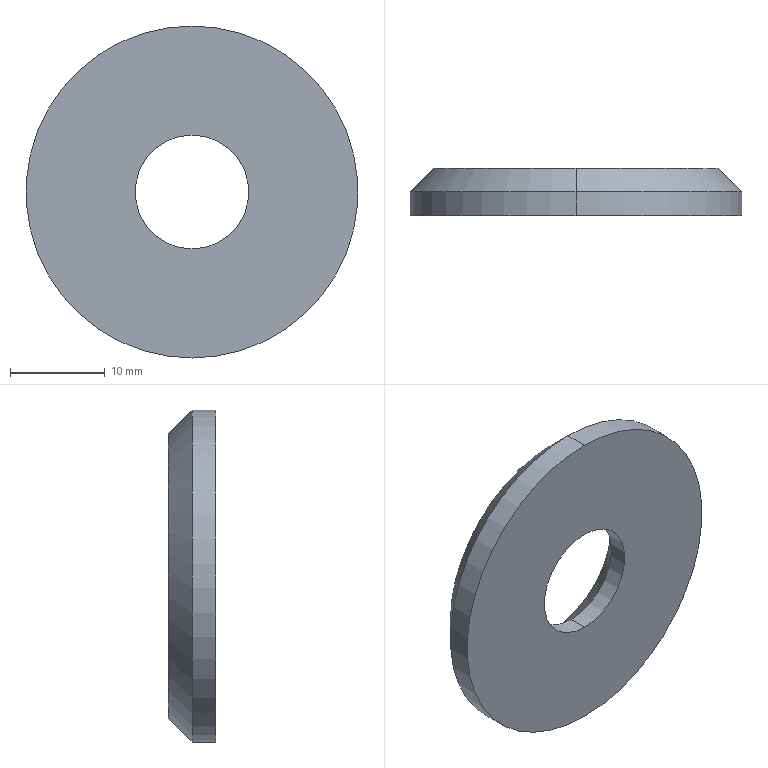Part | SolidWorks | features Chamfer 1, Revolution 1 | 1 solid | 10 faces | box 35 x 5 x 35 mm | volume 3720 mm3 | cone 4 | cylinder 4 | plane 2 | commonest cylinder face diameters 12 x2 35 x2
STEP:
#1=CARTESIAN_POINT('',(0.,7.038,15.));
#2=VERTEX_POINT('',#1);
#3=CARTESIAN_POINT('',(0.,7.038,-15.));
#4=VERTEX_POINT('',#3);
#5=CARTESIAN_POINT('',(0.,7.038,0.));
#6=DIRECTION('',(0.,1.,0.));
#7=DIRECTION('',(0.,0.,-1.));
#8=AXIS2_PLACEMENT_3D('',#5,#6,#7);
#9=CIRCLE('',#8,15.);
#10=EDGE_CURVE('',#2,#4,#9,.T.);
#11=ORIENTED_EDGE('',*,*,#10,.F.);
#12=CARTESIAN_POINT('',(0.,4.538,17.5));
#13=VERTEX_POINT('',#12);
#14=CARTESIAN_POINT('',(0.,7.038,15.));
#15=DIRECTION('',(0.,-0.7071,0.7071));
#16=VECTOR('',#15,1000.);
#17=LINE('',#14,#16);
#18=EDGE_CURVE('',#2,#13,#17,.T.);
#19=ORIENTED_EDGE('',*,*,#18,.T.);
#20=CARTESIAN_POINT('',(0.,4.538,-17.5));
#21=VERTEX_POINT('',#20);
#22=CARTESIAN_POINT('',(0.,4.538,0.));
#23=DIRECTION('',(0.,-1.,0.));
#24=DIRECTION('',(0.,0.,-1.));
#25=AXIS2_PLACEMENT_3D('',#22,#23,#24);
#26=CIRCLE('',#25,17.5);
#27=EDGE_CURVE('',#21,#13,#26,.T.);
#28=ORIENTED_EDGE('',*,*,#27,.F.);
#29=CARTESIAN_POINT('',(0.,7.038,-15.));
#30=DIRECTION('',(0.,-0.7071,-0.7071));
#31=VECTOR('',#30,1000.);
#32=LINE('',#29,#31);
#33=EDGE_CURVE('',#4,#21,#32,.T.);
#34=ORIENTED_EDGE('',*,*,#33,.F.);
#35=EDGE_LOOP('',(#11,#19,#28,#34));
#36=FACE_OUTER_BOUND('',#35,.T.);
#37=CARTESIAN_POINT('',(0.,7.038,0.));
#38=DIRECTION('',(0.,-1.,0.));
#39=DIRECTION('',(0.,0.,-1.));
#40=AXIS2_PLACEMENT_3D('',#37,#38,#39);
#41=CONICAL_SURFACE('',#40,15.,0.7854);
#42=ADVANCED_FACE('',(#36),#41,.T.);
#43=CARTESIAN_POINT('',(0.,2.038,-6.));
#44=VERTEX_POINT('',#43);
#45=CARTESIAN_POINT('',(0.,2.038,6.));
#46=VERTEX_POINT('',#45);
#47=CARTESIAN_POINT('',(0.,2.038,0.));
#48=DIRECTION('',(0.,1.,0.));
#49=DIRECTION('',(0.,0.,1.));
#50=AXIS2_PLACEMENT_3D('',#47,#48,#49);
#51=CIRCLE('',#50,6.);
#52=EDGE_CURVE('',#44,#46,#51,.T.);
#53=ORIENTED_EDGE('',*,*,#52,.F.);
#54=CARTESIAN_POINT('',(0.,4.038,-6.));
#55=VERTEX_POINT('',#54);
#56=CARTESIAN_POINT('',(0.,7.038,-6.));
#57=DIRECTION('',(0.,1.,0.));
#58=VECTOR('',#57,1000.);
#59=LINE('',#56,#58);
#60=EDGE_CURVE('',#44,#55,#59,.T.);
#61=ORIENTED_EDGE('',*,*,#60,.T.);
#62=CARTESIAN_POINT('',(0.,4.038,6.));
#63=VERTEX_POINT('',#62);
#64=CARTESIAN_POINT('',(0.,4.038,0.));
#65=DIRECTION('',(0.,1.,0.));
#66=DIRECTION('',(0.,0.,1.));
#67=AXIS2_PLACEMENT_3D('',#64,#65,#66);
#68=CIRCLE('',#67,6.);
#69=EDGE_CURVE('',#55,#63,#68,.T.);
#70=ORIENTED_EDGE('',*,*,#69,.T.);
#71=CARTESIAN_POINT('',(0.,7.038,6.));
#72=DIRECTION('',(0.,1.,0.));
#73=VECTOR('',#72,1000.);
#74=LINE('',#71,#73);
#75=EDGE_CURVE('',#46,#63,#74,.T.);
#76=ORIENTED_EDGE('',*,*,#75,.F.);
#77=EDGE_LOOP('',(#53,#61,#70,#76));
#78=FACE_OUTER_BOUND('',#77,.T.);
#79=CARTESIAN_POINT('',(0.,7.038,0.));
#80=DIRECTION('',(0.,1.,0.));
#81=DIRECTION('',(0.,0.,1.));
#82=AXIS2_PLACEMENT_3D('',#79,#80,#81);
#83=CYLINDRICAL_SURFACE('',#82,6.);
#84=ADVANCED_FACE('',(#78),#83,.F.);
#85=CARTESIAN_POINT('',(0.,2.038,17.5));
#86=VERTEX_POINT('',#85);
#87=CARTESIAN_POINT('',(0.,2.038,-17.5));
#88=VERTEX_POINT('',#87);
#89=CARTESIAN_POINT('',(0.,2.038,0.));
#90=DIRECTION('',(0.,1.,0.));
#91=DIRECTION('',(0.,0.,1.));
#92=AXIS2_PLACEMENT_3D('',#89,#90,#91);
#93=CIRCLE('',#92,17.5);
#94=EDGE_CURVE('',#86,#88,#93,.T.);
#95=ORIENTED_EDGE('',*,*,#94,.T.);
#96=CARTESIAN_POINT('',(0.,7.038,-17.5));
#97=DIRECTION('',(0.,1.,0.));
#98=VECTOR('',#97,1000.);
#99=LINE('',#96,#98);
#100=EDGE_CURVE('',#88,#21,#99,.T.);
#101=ORIENTED_EDGE('',*,*,#100,.T.);
#102=ORIENTED_EDGE('',*,*,#27,.T.);
#103=CARTESIAN_POINT('',(0.,7.038,17.5));
#104=DIRECTION('',(0.,1.,0.));
#105=VECTOR('',#104,1000.);
#106=LINE('',#103,#105);
#107=EDGE_CURVE('',#86,#13,#106,.T.);
#108=ORIENTED_EDGE('',*,*,#107,.F.);
#109=EDGE_LOOP('',(#95,#101,#102,#108));
#110=FACE_OUTER_BOUND('',#109,.T.);
#111=CARTESIAN_POINT('',(0.,7.038,0.));
#112=DIRECTION('',(0.,1.,0.));
#113=DIRECTION('',(0.,0.,1.));
#114=AXIS2_PLACEMENT_3D('',#111,#112,#113);
#115=CYLINDRICAL_SURFACE('',#114,17.5);
#116=ADVANCED_FACE('',(#110),#115,.T.);
#117=ORIENTED_EDGE('',*,*,#69,.F.);
#118=CARTESIAN_POINT('',(0.,7.038,-9.));
#119=VERTEX_POINT('',#118);
#120=CARTESIAN_POINT('',(0.,7.038,-9.));
#121=DIRECTION('',(0.,0.7071,-0.7071));
#122=VECTOR('',#121,1000.);
#123=LINE('',#120,#122);
#124=EDGE_CURVE('',#55,#119,#123,.T.);
#125=ORIENTED_EDGE('',*,*,#124,.T.);
#126=CARTESIAN_POINT('',(0.,7.038,9.));
#127=VERTEX_POINT('',#126);
#128=CARTESIAN_POINT('',(0.,7.038,0.));
#129=DIRECTION('',(0.,1.,0.));
#130=DIRECTION('',(0.,0.,1.));
#131=AXIS2_PLACEMENT_3D('',#128,#129,#130);
#132=CIRCLE('',#131,9.);
#133=EDGE_CURVE('',#119,#127,#132,.T.);
#134=ORIENTED_EDGE('',*,*,#133,.T.);
#135=CARTESIAN_POINT('',(0.,7.038,9.));
#136=DIRECTION('',(0.,0.7071,0.7071));
#137=VECTOR('',#136,1000.);
#138=LINE('',#135,#137);
#139=EDGE_CURVE('',#63,#127,#138,.T.);
#140=ORIENTED_EDGE('',*,*,#139,.F.);
#141=EDGE_LOOP('',(#117,#125,#134,#140));
#142=FACE_OUTER_BOUND('',#141,.T.);
#143=CARTESIAN_POINT('',(0.,7.038,0.));
#144=DIRECTION('',(0.,1.,0.));
#145=DIRECTION('',(0.,0.,1.));
#146=AXIS2_PLACEMENT_3D('',#143,#144,#145);
#147=CONICAL_SURFACE('',#146,9.,0.7854);
#148=ADVANCED_FACE('',(#142),#147,.F.);
#149=ORIENTED_EDGE('',*,*,#124,.F.);
#150=CARTESIAN_POINT('',(0.,4.038,0.));
#151=DIRECTION('',(0.,1.,0.));
#152=DIRECTION('',(0.,0.,1.));
#153=AXIS2_PLACEMENT_3D('',#150,#151,#152);
#154=CIRCLE('',#153,6.);
#155=EDGE_CURVE('',#63,#55,#154,.T.);
#156=ORIENTED_EDGE('',*,*,#155,.F.);
#157=ORIENTED_EDGE('',*,*,#139,.T.);
#158=CARTESIAN_POINT('',(0.,7.038,0.));
#159=DIRECTION('',(0.,1.,0.));
#160=DIRECTION('',(0.,0.,1.));
#161=AXIS2_PLACEMENT_3D('',#158,#159,#160);
#162=CIRCLE('',#161,9.);
#163=EDGE_CURVE('',#127,#119,#162,.T.);
#164=ORIENTED_EDGE('',*,*,#163,.T.);
#165=EDGE_LOOP('',(#149,#156,#157,#164));
#166=FACE_OUTER_BOUND('',#165,.T.);
#167=CARTESIAN_POINT('',(0.,7.038,0.));
#168=DIRECTION('',(0.,1.,0.));
#169=DIRECTION('',(0.,0.,1.));
#170=AXIS2_PLACEMENT_3D('',#167,#168,#169);
#171=CONICAL_SURFACE('',#170,9.,0.7854);
#172=ADVANCED_FACE('',(#166),#171,.F.);
#173=CARTESIAN_POINT('',(0.,7.038,0.));
#174=DIRECTION('',(0.,1.,0.));
#175=DIRECTION('',(0.,0.,-1.));
#176=AXIS2_PLACEMENT_3D('',#173,#174,#175);
#177=CIRCLE('',#176,15.);
#178=EDGE_CURVE('',#4,#2,#177,.T.);
#179=ORIENTED_EDGE('',*,*,#178,.T.);
#180=ORIENTED_EDGE('',*,*,#10,.T.);
#181=EDGE_LOOP('',(#179,#180));
#182=FACE_OUTER_BOUND('',#181,.T.);
#183=ORIENTED_EDGE('',*,*,#163,.F.);
#184=ORIENTED_EDGE('',*,*,#133,.F.);
#185=EDGE_LOOP('',(#183,#184));
#186=FACE_BOUND('',#185,.T.);
#187=CARTESIAN_POINT('',(9.,7.038,0.));
#188=DIRECTION('',(0.,-1.,0.));
#189=DIRECTION('',(0.,0.,-1.));
#190=AXIS2_PLACEMENT_3D('',#187,#188,#189);
#191=PLANE('',#190);
#192=ADVANCED_FACE('',(#182,#186),#191,.F.);
#193=ORIENTED_EDGE('',*,*,#100,.F.);
#194=CARTESIAN_POINT('',(0.,2.038,0.));
#195=DIRECTION('',(0.,1.,0.));
#196=DIRECTION('',(0.,0.,1.));
#197=AXIS2_PLACEMENT_3D('',#194,#195,#196);
#198=CIRCLE('',#197,17.5);
#199=EDGE_CURVE('',#88,#86,#198,.T.);
#200=ORIENTED_EDGE('',*,*,#199,.T.);
#201=ORIENTED_EDGE('',*,*,#107,.T.);
#202=CARTESIAN_POINT('',(0.,4.538,0.));
#203=DIRECTION('',(0.,-1.,0.));
#204=DIRECTION('',(0.,0.,-1.));
#205=AXIS2_PLACEMENT_3D('',#202,#203,#204);
#206=CIRCLE('',#205,17.5);
#207=EDGE_CURVE('',#13,#21,#206,.T.);
#208=ORIENTED_EDGE('',*,*,#207,.T.);
#209=EDGE_LOOP('',(#193,#200,#201,#208));
#210=FACE_OUTER_BOUND('',#209,.T.);
#211=CARTESIAN_POINT('',(0.,7.038,0.));
#212=DIRECTION('',(0.,1.,0.));
#213=DIRECTION('',(0.,0.,1.));
#214=AXIS2_PLACEMENT_3D('',#211,#212,#213);
#215=CYLINDRICAL_SURFACE('',#214,17.5);
#216=ADVANCED_FACE('',(#210),#215,.T.);
#217=ORIENTED_EDGE('',*,*,#94,.F.);
#218=ORIENTED_EDGE('',*,*,#199,.F.);
#219=EDGE_LOOP('',(#217,#218));
#220=FACE_OUTER_BOUND('',#219,.T.);
#221=CARTESIAN_POINT('',(0.,2.038,0.));
#222=DIRECTION('',(0.,1.,0.));
#223=DIRECTION('',(0.,0.,1.));
#224=AXIS2_PLACEMENT_3D('',#221,#222,#223);
#225=CIRCLE('',#224,6.);
#226=EDGE_CURVE('',#46,#44,#225,.T.);
#227=ORIENTED_EDGE('',*,*,#226,.T.);
#228=ORIENTED_EDGE('',*,*,#52,.T.);
#229=EDGE_LOOP('',(#227,#228));
#230=FACE_BOUND('',#229,.T.);
#231=CARTESIAN_POINT('',(17.5,2.038,0.));
#232=DIRECTION('',(0.,1.,0.));
#233=DIRECTION('',(0.,0.,1.));
#234=AXIS2_PLACEMENT_3D('',#231,#232,#233);
#235=PLANE('',#234);
#236=ADVANCED_FACE('',(#220,#230),#235,.F.);
#237=ORIENTED_EDGE('',*,*,#60,.F.);
#238=ORIENTED_EDGE('',*,*,#226,.F.);
#239=ORIENTED_EDGE('',*,*,#75,.T.);
#240=ORIENTED_EDGE('',*,*,#155,.T.);
#241=EDGE_LOOP('',(#237,#238,#239,#240));
#242=FACE_OUTER_BOUND('',#241,.T.);
#243=CARTESIAN_POINT('',(0.,7.038,0.));
#244=DIRECTION('',(0.,1.,0.));
#245=DIRECTION('',(0.,0.,1.));
#246=AXIS2_PLACEMENT_3D('',#243,#244,#245);
#247=CYLINDRICAL_SURFACE('',#246,6.);
#248=ADVANCED_FACE('',(#242),#247,.F.);
#249=ORIENTED_EDGE('',*,*,#18,.F.);
#250=ORIENTED_EDGE('',*,*,#178,.F.);
#251=ORIENTED_EDGE('',*,*,#33,.T.);
#252=ORIENTED_EDGE('',*,*,#207,.F.);
#253=EDGE_LOOP('',(#249,#250,#251,#252));
#254=FACE_OUTER_BOUND('',#253,.T.);
#255=CARTESIAN_POINT('',(0.,7.038,0.));
#256=DIRECTION('',(0.,-1.,0.));
#257=DIRECTION('',(0.,0.,-1.));
#258=AXIS2_PLACEMENT_3D('',#255,#256,#257);
#259=CONICAL_SURFACE('',#258,15.,0.7854);
#260=ADVANCED_FACE('',(#254),#259,.T.);
#261=CLOSED_SHELL('',(#42,#84,#116,#148,#172,#192,#216,#236,#248,#260));
#262=MANIFOLD_SOLID_BREP('',#261);
#263=CARTESIAN_POINT('',(0.,0.,0.));
#264=DIRECTION('',(0.,0.,1.));
#265=DIRECTION('',(1.,0.,0.));
#266=AXIS2_PLACEMENT_3D('',#263,#264,#265);
#267=(LENGTH_UNIT()NAMED_UNIT(*)SI_UNIT(.MILLI.,.METRE.));
#268=UNCERTAINTY_MEASURE_WITH_UNIT(LENGTH_MEASURE(0.00001),#267,'','');
#269=(NAMED_UNIT(*)PLANE_ANGLE_UNIT()SI_UNIT($,.RADIAN.));
#270=(NAMED_UNIT(*)SI_UNIT($,.STERADIAN.)SOLID_ANGLE_UNIT());
#271=(GEOMETRIC_REPRESENTATION_CONTEXT(3)GLOBAL_UNCERTAINTY_ASSIGNED_CONTEXT((#268))GLOBAL_UNIT_ASSIGNED_CONTEXT((#267,#269,#270))REPRESENTATION_CONTEXT('',''));
#272=ADVANCED_BREP_SHAPE_REPRESENTATION('',(#262,#266),#271);